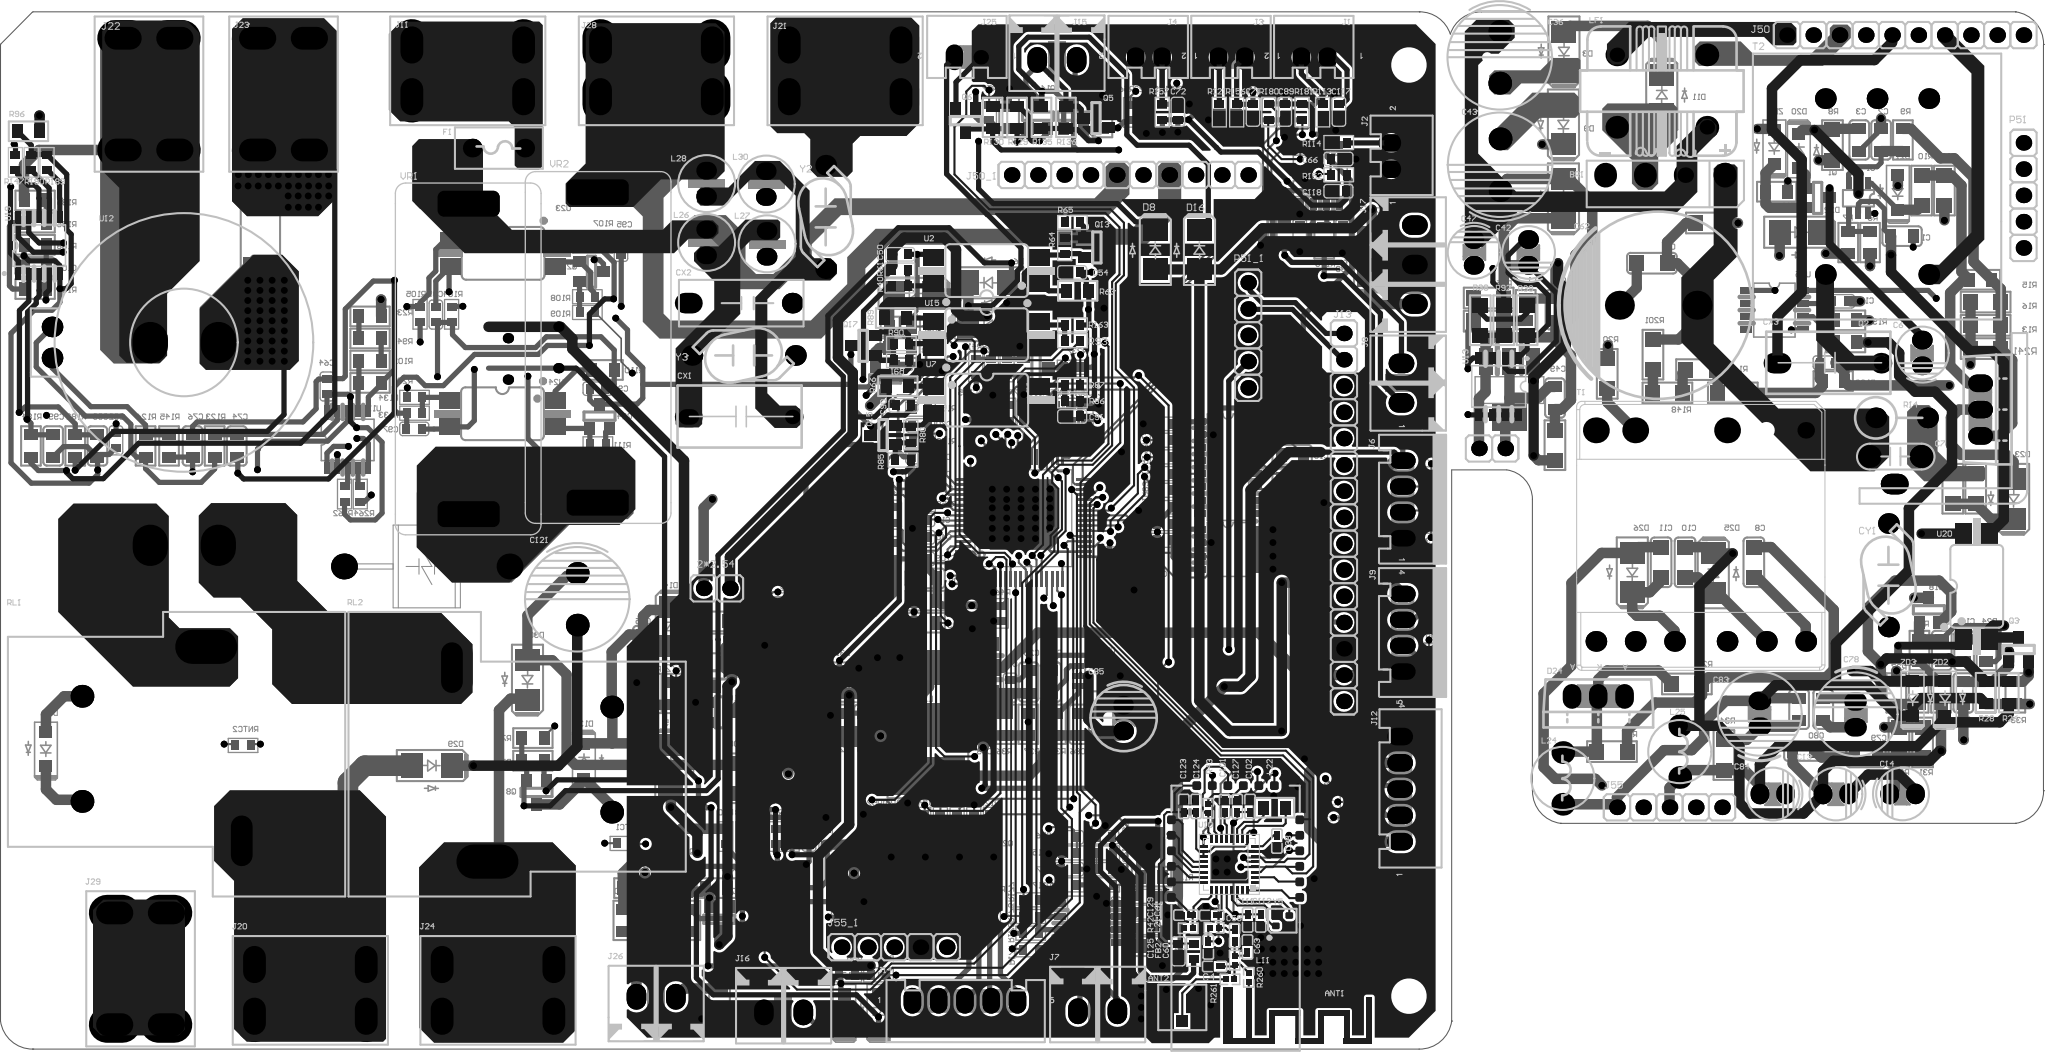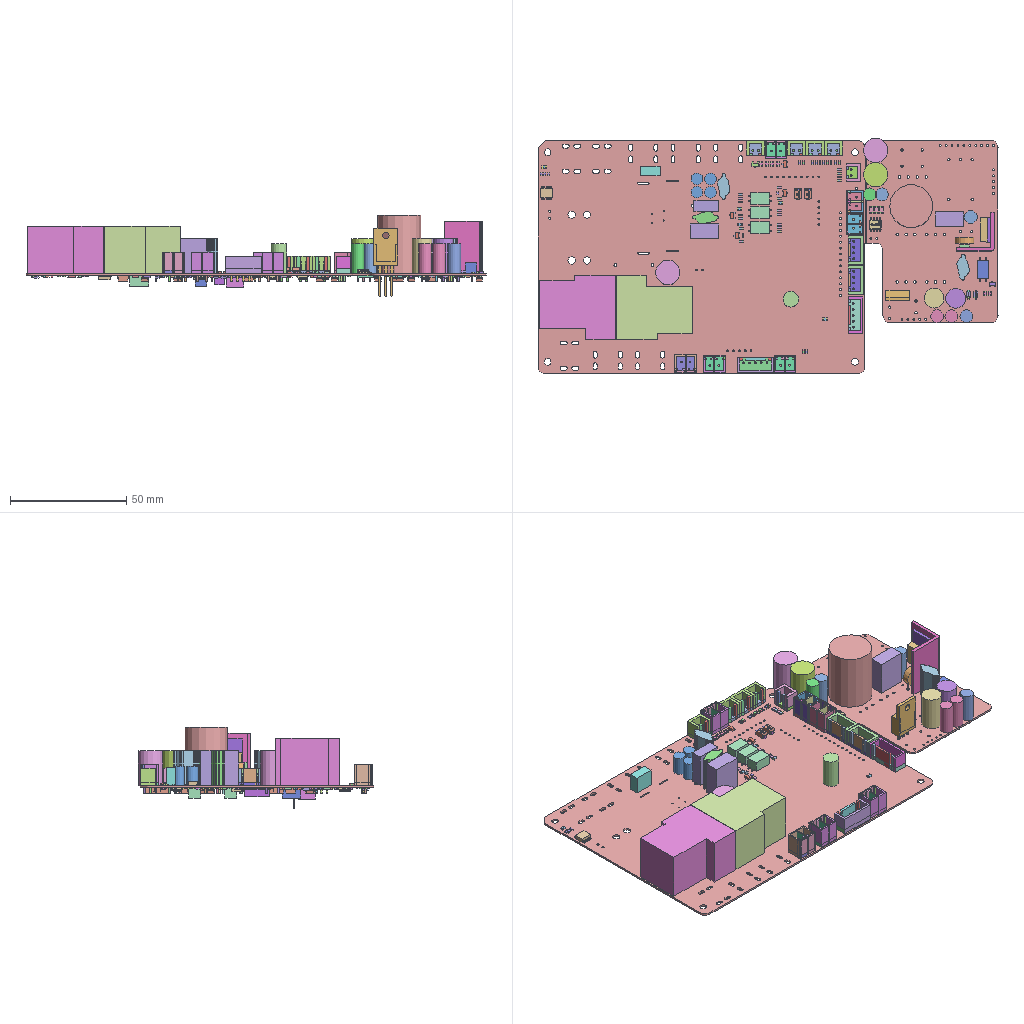Circuit board layout | Altium Designer | box 197.5 x 101.1 x 34.9 mm
Layer stack:
# Altium Designer layer stack of  (unit mm; dielectric type: 0 none, 1 core, 2 prepreg, 3 surface material)
index,name,kind,layer,copper_thickness_mm,dielectric_type,dielectric_thickness_mm,dielectric_material,dielectric_constant
0,Top Paste,other,,,,,,
1,Top Overlay,other,,,,,,
2,Top Solder,dielectric,,,3,0.0102,Solder Resist,3.5
3,Top Layer,copper,Top Layer,0.0356,,,,
4,Dielectric 1,dielectric,,,1,0.254,FR-4,4.2
5,02,copper,02,0.036,,,,
6,Dielectric 6,dielectric,,,2,0.127,,4.2
7,03,copper,03,0.036,,,,
8,Dielectric 5,dielectric,,,1,0.254,,4.2
9,Bottom Layer,copper,Bottom Layer,0.0356,,,,
10,Bottom Solder,dielectric,,,3,0.0102,Solder Resist,3.5
11,Bottom Overlay,other,,,,,,
12,Bottom Paste,other,,,,,,
# drill layer pairs: low layer,high layer
drill_pair,Top Layer,Bottom Layer
Part placement:
Designator,Comment,Layer,Footprint,Center-X(mm),Center-Y(mm),Rotation
,Comment,TopLayer,蓝牙,49.246,-30.063,270
P51_1,(2.54 socket),TopLayer,P5-2.54,50.463,18.866,270
J55_1,(2.54 socket),TopLayer,P5-2.54,16.251,-40.278,0
J50_1,Header -10-2.54,TopLayer,p10-2.54,39.033,34.36,0
2*2.54,Comment,TopLayer,p2-2.54,-0.8962,-5.594,180
,Comment,TopLayer,p2-2.54,74.041,7.925,180
R148,2.4M,BottomLayer,R1206-T,90.985,13.293,180
R241,1.5R,BottomLayer,R1206-T,121.742,17.577,180
R93,100R,TopLayer,R0603-T,33.48,18.339,180
CX2,0.33uF,TopLayer,CX10.0X4.0-P7.5,1.397,21.971,180
C4,0.5pF/50V,TopLayer,C0402-T,47.221,-42.139,180
J13,(2.54 socket),TopLayer,P15-2.54,59.718,1.262,0
Y3,2.2nF/400V,TopLayer,CY7.5X4.7_P10_AI-DS,1.702,16.916,90
Y2,2.2nF/400V,TopLayer,CY7.5X4.7_P10_AI-DS,9.627,30.302,0
J22,Terminal,TopLayer,接线端子（12X9mm）,-55.778,42.175,270
D16,RS1D,TopLayer,SMA,45.745,27.127,90
D8,RS1D,TopLayer,SMA,41.478,27.127,90
D7,RS1D,BottomLayer,SMA,62.182,26.459,270
T2,EFD30,TopLayer,变压器,111.248,33.24,180
U10,TLSR8251,TopLayer,QFN32_5X5MM,48.643,-32.271,180
L1,1mH  DR8*10,BottomLayer,R0805-T,77.289,21.339,90
U26,MAX232,BottomLayer,SO-16-T,48.516,6.114,270
U13,OB222*,TopLayer,SO-8-t,74.676,13.919,180
D11,US1M,BottomLayer,SMA,90.449,42.139,90
D9,MUR406,BottomLayer,SMA,80.924,39.218,270
D4,MUR406,BottomLayer,SMA,80.924,32.075,270
D3,US1M,BottomLayer,SMA,80.975,46.279,270
C47,100uF/16V,TopLayer,CE5-P2.5MM-AI,71.611,26.873,90
C42,10uF/50V,TopLayer,CE5-P2.5MM-AI,78.259,26.873,270
U8,AT403ARC,BottomLayer,so-64-t1,28.755,1.207,270
C43,100uF/25V,TopLayer,CE10-P5.0MM-AI,75.417,35.347,270
C36,10uF/400V,TopLayer,CE10-P5.0MM-AI,74.172,45.731,90
ZD3,12V,TopLayer,SOD-123-T,114.683,-16.219,270
ZD2,6.2V,TopLayer,SOD-123-T,117.808,-16.219,270
ZD1,13V,BottomLayer,SOD-123-T,101.323,37.07,270
ZC1,Discharge tube SE801H-L,BottomLayer,ZC_8X6.5__P:16.0mm,-28.931,-3.48,0
Y5,24MHz,TopLayer,23047-00020-11_32M_SMD¾§Õñ,53.787,-37.716,0
Y1,25MHz,BottomLayer,SMD晶振（HC-49）,12.954,0,270
U25,LM293,BottomLayer,so-8-t,101.323,21.298,270
U24,BPC-1009,BottomLayer,OPT-SMT(LTV-817S),-21.613,11.281,180
U23,BPC-1009,BottomLayer,OPT-SMT(LTV-817S),-21.552,26.784,180
U22,RS485,BottomLayer,SO-8-T,34.996,-37.947,90
U20,LTV-817C,TopLayer,OPT-SMT(LTV-817S),120.881,-5.397,90
U19,BL0942,TopLayer,SO-10-T（脚距1.0mm),-66.396,27.534,0
U18,TL431,BottomLayer,SOT-23((TL431)(A_K_R)-T,116.258,-7.683,180
U17,SM8102H,BottomLayer,SOT-23-6-T,35.514,-14.046,270
U16,AMS1117-3V3,BottomLayer,SOT-223-T,75.717,13.619,0
U15,BPC-1009,TopLayer,OPT-SMT(LTV-817S),25.197,18.923,0
U14,LM2904,BottomLayer,so-8-t,4.32,-37.274,180
U12,CTZ-LB-10,TopLayer,23012-00041-10__µçÁ÷»¥¸ÐÆ÷,-65.149,18.172,270
U11,BL0942,BottomLayer,SO-10-T（脚距1.0mm),-36.574,8.75,0
U9,AT24C16M/TR,BottomLayer,SO-8-t,48.516,-1.839,270
U7,BPC-1009,TopLayer,OPT-SMT(LTV-817S),25.197,12.598,0
U6,TJA1050,BottomLayer,SO-8-T,57.432,34.27,0
U5,AMS1117-3V3,BottomLayer,SOT-223-T,22.358,-13.271,270
U3,TLP785,BottomLayer,OPT-SMT(LTV-817S),4.981,-14.77,90
U2,BPC-1009,TopLayer,OPT-SMT(LTV-817S),25.197,25.118,180
U1,OB2365E,BottomLayer,SOT-23-6-T,109.449,32.101,180
T1,PQ20/20,TopLayer,PQ2020,94.211,-0.5206,0
RNTC2,NTC,BottomLayer,R0603-t,-46.685,-20.777,0
RNTC1,NTC,BottomLayer,R0603-t,-9.779,-30.251,180
RL2,T9VV1K15-12S,TopLayer,继电器（T9VV1K15-12S）,-18.774,-22.632,90
RL1,T9VV1K15-12S,TopLayer,继电器（T9VV1K15-12S）,-54.532,-20.622,270
R264,10K,BottomLayer,R0603-T,-35.354,3.518,90
R263,30K,BottomLayer,R1206-T,6.056,-23.952,90
R261,0R,TopLayer,R0402-T,48.706,-43.384,180
R260,0R,TopLayer,R0402-T,50.523,-43.194,90
R240,10K,BottomLayer,R0603-T,14.731,-42.95,0
R239,10K,BottomLayer,R0603-T,27.162,15.799,90
R238,100R,BottomLayer,R0603-T,25.646,15.799,90
R237,3K,BottomLayer,R0603-T,33.445,15.773,180
R236,100R,BottomLayer,R0603-T,60.792,-24.651,180
R235,100R,BottomLayer,R0603-T,60.792,-26.2,180
R234,100R,BottomLayer,R0603-T,60.792,-27.749,180
R233,10K,BottomLayer,R0603-T,60.792,-23.101,180
R232,1k,BottomLayer,R0805-T,-34.412,14.262,0
R231,1.5M,BottomLayer,R0805-T,-34.412,20.689,0
R214,5.1K,BottomLayer,R0603-T,24.314,-36.541,90
R213,5.1K,BottomLayer,R0603-T,22.79,-36.534,90
R201,2.4M,BottomLayer,R1206-T,89.585,16.993,90
R200,30K,BottomLayer,R1206-T,1.145,-23.952,90
R199,2K,BottomLayer,R0805-T,19.245,-8.915,180
R198,30K,BottomLayer,R1206-T,3.601,-23.952,270
R197,1K,BottomLayer,R0805-T,19.245,-6.782,180
R196,10K,BottomLayer,R0805-T,5.182,-7.391,0
R195,30K,BottomLayer,R1206-T,8.511,-23.952,90
R194,20K,BottomLayer,R0805-T,108.201,18.174,180
R193,1K,BottomLayer,R0805-T,108.201,20.308,0
R192,22K,BottomLayer,R0805-T,107.008,14.44,180
R191,2.4M,BottomLayer,R1206-T,97.307,13.293,180
R190,10K,TopLayer,R0603-T,-67.157,35.579,270
R189,10K,TopLayer,R0603-T,-65.633,35.579,270
R188,1k,BottomLayer,R0805-T,-66.782,27.614,180
R187,1.5M,BottomLayer,R0805-T,-66.782,23.334,180
R186,1.5M,BottomLayer,R0805-T,-66.782,29.754,0
R185,1.5M,BottomLayer,R0805-T,-66.782,31.894,180
R184,1k,BottomLayer,R0805-T,-67.187,8.17,90
R183,1mΩ,BottomLayer,R2512-T,-45.009,28.626,270
R182,1k,BottomLayer,R0805-T,-62.907,8.17,90
R181,100R,TopLayer,R0603-T,55.677,40.437,270
R180,100R,TopLayer,R0603-T,52.451,40.437,90
R179,120R,BottomLayer,R0805-T,57.813,28.185,90
R178,10K,BottomLayer,R0603-T,40.615,-35.36,180
R177,100R,BottomLayer,R0603-T,29.445,-35.703,0
R176,120R,BottomLayer,R0805-T,41.122,-33.455,0
R175,100R,BottomLayer,R0603-T,29.445,-37.312,0
R174,100R,BottomLayer,R0603-T,29.445,-40.529,0
R173,10K,BottomLayer,R0603-T,29.445,-38.92,0
R171,10K,BottomLayer,R0603-T,40.615,-36.884,0
R170,0R,BottomLayer,R0603-T,68.176,4.724,270
R163,4.7K,TopLayer,R0603-T,33.48,19.86,0
R162,10K,BottomLayer,R0603-T,-36.878,3.518,270
R159,NC,BottomLayer,R0603-T,42.171,40.41,90
R158,1K,BottomLayer,R0603-T,18.796,2.514,0
R157,1K,TopLayer,R0603-T,42.16,40.436,270
R156,NC,TopLayer,R0603-T,49.352,40.437,90
R155,1K,BottomLayer,R0603-T,18.796,11.723,0
R154,10K,BottomLayer,R0603-T,50.922,40.437,270
R153,1K,BottomLayer,R0603-T,18.796,8.653,0
R152,10K,TopLayer,R0603-T,59.217,34.377,0
R151,1K,BottomLayer,R0603-T,31.834,11.349,270
R150,10K,BottomLayer,R0603-T,55.667,40.437,270
R149,2.4M,BottomLayer,R1206-T,94.234,15.545,180
R147,10K,TopLayer,R0603-T,-68.681,35.579,90
R145,1.2K,BottomLayer,R0805-T,-53.84,8.17,90
R142,NC,BottomLayer,RES/0603,42.446,7.11,180
R141,NC,BottomLayer,RES/0603,42.446,8.722,180
R140,0R,BottomLayer,R0805-T,68.478,-7.67,90
R139,0R,BottomLayer,R0805-T,68.478,-12.802,270
R137,0R,BottomLayer,R0603-T,68.176,1.161,90
R136,10K,TopLayer,R0805-T,32.849,39.929,270
R135,5.1K,TopLayer,R0805-T,30.487,39.929,270
R134,100R,BottomLayer,R0603-T,-30.112,12.865,0
R133,4.7K,BottomLayer,R0603-T,-30.112,11.334,180
R130,10K,TopLayer,R0805-T,25.762,39.929,90
R129,5.1K,TopLayer,R0805-T,28.124,39.929,90
R128,10K,BottomLayer,R0603-T,23.94,-28.188,90
R127,100R,BottomLayer,R0603-T,25.552,-28.188,90
R126,5.1K,BottomLayer,R0603-T,25.838,-36.541,90
R125,5.1K,BottomLayer,R0603-T,21.271,-36.541,90
R124,1.2k,BottomLayer,R0805-T,-56.109,8.17,90
R123,1.2K,BottomLayer,R0805-T,-49.432,8.17,270
R122,1K,BottomLayer,R0603-T,40.617,40.41,270
R121,1K,TopLayer,R0603-T,47.676,40.437,270
R120,1K,BottomLayer,R0603-T,36.599,-34.255,0
R119,1K,BottomLayer,R0603-T,30.325,11.349,270
R118,10K,BottomLayer,R0603-T,36.599,-31.17,0
R117,1K,BottomLayer,R0603-T,33.181,-34.255,180
R116,1K,BottomLayer,R0603-T,27.306,11.349,270
R115,10K,BottomLayer,R0603-T,33.181,-31.17,180
R114,1K,TopLayer,R0603-T,59.217,37.49,0
R113,1K,TopLayer,R0603-T,57.658,40.437,90
R112,2K,BottomLayer,R0603-T,-12.391,6.845,180
R111,4.7K,BottomLayer,R0603-T,-12.391,8.369,180
R110,300R,BottomLayer,R0805-T,-11.885,15.513,180
R109,2K,BottomLayer,R0603-T,-13.407,21.069,180
R108,4.7K,BottomLayer,R0603-T,-13.407,22.593,0
R107,470R,BottomLayer,R0805-T,-12.901,27.8,0
R105,100R,BottomLayer,R0603-T,-29.578,20.891,270
R104,4.7K,BottomLayer,R0603-T,-26.53,20.891,270
R103,10K,BottomLayer,R0805-T,-8.913,-34.565,0
R102,1.5M,BottomLayer,R0805-T,-34.412,16.421,0
R100,510K,BottomLayer,R0805-T,-9.929,-37.689,90
R99,1K,BottomLayer,R0805-T,-5.611,-37.689,90
R97,1K,BottomLayer,R0805-T,-3.452,-37.689,270
R96,0R,TopLayer,R0805-T,-67.425,38.583,180
R95,1.2K,BottomLayer,R1206-T,80.112,8.243,90
R94,1.5M,BottomLayer,R0805-T,-34.412,18.555,180
R92,390K,TopLayer,R1206-T,75.159,20.32,90
R91,2K,TopLayer,R0603-T,16.942,16.434,0
R90,4.7K,TopLayer,R0603-T,16.942,18.059,0
R89,470R,TopLayer,R0805-T,16.384,20.531,0
R88,2R,BottomLayer,R1206-T,73.707,20.231,180
R87,100R,TopLayer,R0603-T,33.48,14.072,180
R86,4.7K,TopLayer,R0603-T,33.48,12.533,0
R85,2K,TopLayer,R0603-T,17.11,6.807,0
R84,10K,BottomLayer,R0603-T,3.179,-29.584,270
R83,100R,BottomLayer,RES/0603,42.446,3.885,0
R82,10K,BottomLayer,R0603-T,6.386,-29.584,90
R81,10K,BottomLayer,R0603-T,4.783,-29.584,270
R80,4.7K,TopLayer,R0603-T,17.86,9.22,90
R79,1.5K,BottomLayer,R0603-T,11.613,-35.877,180
R78,124K,BottomLayer,R0603-T,1.626,-29.584,270
R77,10K,BottomLayer,R0603-T,11.613,-34.38,0
R75,2K,BottomLayer,R0805-T,-0.9398,-34.565,180
R74,10K,BottomLayer,R0805-T,-18.672,-22.254,180
R73,10K,BottomLayer,R0805-T,-7.186,-15.751,270
R71,470R,BottomLayer,R0805-T,-18.672,-20.067,0
R70,5.1K,BottomLayer,R0805-T,-0.8636,-10.922,180
R69,10K,BottomLayer,R0805-T,-0.889,-8.788,180
R68,10K,BottomLayer,R0805-T,16.815,17.628,180
R67,470R,BottomLayer,R0805-T,16.84,19.71,0
R66,470R,TopLayer,R0805-T,16.603,13.945,0
R65,2K,TopLayer,R0603-T,33.48,29.766,0
R64,4.7K,TopLayer,R0603-T,32.73,27.51,270
R63,470R,TopLayer,R0805-T,33.986,23.162,0
R61,4.7K,TopLayer,R0603-T,16.794,25.167,180
R60,100R,BottomLayer,R0603-T,-0.0281,-29.584,90
R59,10K,BottomLayer,R0805-T,27.358,39.904,270
R58,10K,BottomLayer,R0805-T,36.375,39.904,270
R57,1K,BottomLayer,R0603-T,25.453,40.41,90
R56,1K,BottomLayer,R0603-T,39.093,40.41,270
R55,10K,BottomLayer,R0603-T,11.669,-42.95,180
R54,10K,BottomLayer,R0603-T,42.446,0.6601,0
R53,10K,BottomLayer,R0603-T,42.446,-0.9524,0
R52,10K,BottomLayer,R0603-T,14.267,-28.188,90
R51,100R,BottomLayer,R0603-T,15.879,-28.188,90
R50,10K,BottomLayer,R0603-T,20.715,-28.188,90
R49,10K,BottomLayer,R0603-T,17.491,-28.188,90
R48,100R,BottomLayer,R0603-T,22.328,-28.188,90
R47,100R,BottomLayer,R0603-T,19.103,-28.188,90
R46,10K,BottomLayer,R0603-T,26.594,-8.013,270
R45,2R,BottomLayer,R1206-T,73.707,22.468,180
R44,1M,BottomLayer,R0603-T,8.788,-0.0508,90
R43,1K,TopLayer,R0402-T,46.611,-26.858,270
R42,0R,TopLayer,R0402-T,44.667,-38.445,0
R41,5.1K,BottomLayer,R0603-T,24.131,15.799,90
R40,100R,TopLayer,R0603-T,16.794,23.643,180
R39,390K,TopLayer,R1206-T,77.419,20.32,90
R38,390K,TopLayer,R1206-T,72.898,20.32,270
R37,22K1,BottomLayer,R0805-T,29.212,-18.732,90
R36,100K,BottomLayer,R0805-T,27.053,-18.732,270
R35,10K,BottomLayer,R0805-T,31.879,-18.732,90
R34,N.C,BottomLayer,R1206-T,96.446,-21.704,270
R33,470R,BottomLayer,R0805-T,124.612,-15.697,90
R32,1K1,BottomLayer,R0805-T,121.745,-15.697,270
R31,N.C,BottomLayer,R1206-T,115.649,-20.489,90
R30,N.C,BottomLayer,R1206-T,113.363,-20.489,90
R29,200K,BottomLayer,R0805-T,113.109,-15.702,90
R28,6K8,TopLayer,R0805-T,121.742,-15.672,90
R27,1K8,BottomLayer,R0805-T,115.268,-15.702,90
R26,N.A,TopLayer,R0805-T,123.977,-15.672,90
R25,470R,BottomLayer,R0805-T,117.427,-15.702,90
R24,N.C,BottomLayer,R0805-T,121.821,-11.603,90
R23,22R,BottomLayer,R1206-T,92.865,-14.834,180
R22,22R,BottomLayer,R1206-T,85.626,-21.374,180
R21,4K7,BottomLayer,R0805-T,115.344,-11.603,90
R20,2.2R,BottomLayer,R1206-T,85.166,15.138,270
R19,100R,BottomLayer,R1206-T,120.779,4.035,90
R18,NC,BottomLayer,RES/0603,42.446,5.497,0
R17,100R,BottomLayer,R1206-T,118.57,4.035,90
R16,1.5R,BottomLayer,R1206-T,121.742,22.073,180
R15,10K,BottomLayer,R0805-T,121.242,24.232,0
R14,100K 1W,TopLayer,R-1W-P5.0-V,113.627,10.884,0
R13,1.5R,BottomLayer,R1206-T,121.742,19.825,180
R12,10R,BottomLayer,R1206-T,117.757,32.851,90
R11,10K,BottomLayer,R0805-T,101.547,32.744,180
R10,47R,BottomLayer,R1206-T,115.547,32.851,90
R9,470R,BottomLayer,R0805-T,113.744,37.745,90
R8,220K,BottomLayer,R1206-T,106.936,37.245,90
R7,27K,BottomLayer,R0805-T,108.46,27.825,270
R6,100K,BottomLayer,R0805-T,110.569,27.826,90
R5,220K,BottomLayer,R1206-T,95.185,29.718,0
Q24,MMBT4403LT1G,BottomLayer,SOT-23-T,-12.235,11.036,180
Q23,MMBT4403LT1G,BottomLayer,SOT-23-T,-13.024,25.006,90
Q22,AP2306AGN,BottomLayer,SOT-23-T,29.947,15.723,90
Q21,AP2306AGN,BottomLayer,SOT-23-T,24.917,-31.737,0
Q20,AP2306AGN,BottomLayer,SOT-23-T,15.011,-31.737,0
Q19,AP2306AGN,BottomLayer,SOT-23-T,21.615,-31.737,0
Q18,AP2306AGN,BottomLayer,SOT-23-T,18.313,-31.737,0
Q17,MMBT4403LT1G,TopLayer,SOT-23-T,13.252,17.846,90
Q16,AOSS21311C,BottomLayer,SOT-23-T,33.581,40.027,180
Q15,MMBT4403LT1G,TopLayer,SOT-23-T,15.18,9.22,90
Q14,AOSS21311C,BottomLayer,SOT-23-T,30.152,40.027,180
Q13,MMBT4403LT1G,TopLayer,SOT-23-T,35.826,27.353,270
Q12,LMBT5401LT1G,BottomLayer,SOT-23-T,-4.722,-33.738,180
Q11,LMBT5551LT1G,BottomLayer,SOT-23-T,-0.658,-37.566,0
Q10,AP2306AGN,BottomLayer,SOT-23-T,-0.6604,-17.577,90
Q9,AOSS21311C,BottomLayer,SOT-23-T,-1.016,-13.945,0
Q8,AP2306AGN,BottomLayer,SOT-23-T,-18.322,-25.302,0
Q7,AP2306AGN,BottomLayer,SOT-23-T,15.367,14.656,0
Q6,AP2306AGN,TopLayer,SOT-23-T,23.171,39.626,180
Q5,AP2306AGN,TopLayer,SOT-23-T,35.77,39.853,90
Q3,2N3904,TopLayer,SOT-23-T,124.945,-11.519,0
Q2,4A/650V,TopLayer,TO-220((É¢ÈÈÆ¬16.5X16mm_ºñ1.5mm),117.106,9.353,270
Q1,BC846B,BottomLayer,SOT-23-T,105.489,32.144,90
LF1,18mH,TopLayer,UU9.8_-_(8.7MM),90.449,42.469,0
L31,3.9uH,BottomLayer,R0805-T,10.95,-14.655,90
L30,100uH,TopLayer,71453-00013-11_(5X8.3_P:2.5),3.886,33.483,270
L29,SWCS0503-100MT 10uH/1.8A,BottomLayer,L(8x8x4)-3d,19.507,-21.374,90
L28,100uH,TopLayer,71453-00013-11_(5X8.3_P:2.5),-1.88,33.528,270
L27,100uH,TopLayer,71453-00013-11_(5X8.3_P:2.5),3.962,27.706,270
L26,100uH,TopLayer,71453-00013-11_(5X8.3_P:2.5),-1.88,27.838,270
L25,3.3uH,TopLayer,L-DR6-P5.0,92.179,-21.374,270
L24,3.3uH,TopLayer,L-DR6-P5.0,80.876,-23.965,270
L22,47uH,TopLayer,R0805-T,53.018,-26.797,180
L21,1.3nH,TopLayer,R0402-T,47.166,-38.406,0
L11,3.3nH,TopLayer,R0402-T,49.151,-41.529,90
J29,Terminal,TopLayer,接线端子（12X9mm）,-56.591,-42.367,90
J28,Terminal,TopLayer,接线端子（12X9mm）,-6.731,44.425,0
J26,CON2,TopLayer,CON2-3.81,-6.757,-45.072,180
J25,CON2,TopLayer,con2-2.54,23.345,45.733,180
J24,Terminal,TopLayer,接线端子（12X9mm）,-22.045,-44.452,180
J23,Terminal,TopLayer,接线端子（12X9mm）,-42.774,42.175,270
J21,Terminal,TopLayer,接线端子（12X9mm）,11.506,44.425,0
J20,Terminal,TopLayer,接线端子（12X9mm）,-40.18,-44.452,0
J17,CON3,TopLayer,CON3-3.81,66.576,25.697,90
J16,CON2,TopLayer,CON2-3.81,5.562,-46.582,0
J15,CON2,TopLayer,CON2-3.81,31.981,45.479,0
J14,CON5,TopLayer,CON5-2.54,23.088,-45.453,0
J12,CON5,TopLayer,CON5-2.54,65.153,-25.001,90
J11,Terminal,TopLayer,接线端子（12X9mm）,-24.968,44.425,180
J9,CON4,TopLayer,CON4-2.5,65.407,-9.888,270
J8,CON2,TopLayer,CON2-3.81,65.28,14.242,270
J7,CON2,TopLayer,CON2-3.81,35.915,-46.469,0
J6,CON4,TopLayer,CON4-2.5,65.407,2.999,270
J4,CON2,TopLayer,CON2-2.54,40.871,45.733,180
J3,CON2,TopLayer,CON2-2.54,48.872,45.733,180
J2,CON2,TopLayer,CON2-2.54,64.29,36.187,90
J1,CON2,TopLayer,CON2-2.54,56.873,45.733,180
FB2,BLM15HG102SN1,TopLayer,R0603-T,45.189,-40.703,90
FB1,600Ω/100MHZ,BottomLayer,R1206-T,-0.6326,-45.733,90
F1,T2A/250V,TopLayer,FUSE-TE5,-21.996,36.957,180
D31,1N4148,BottomLayer,SOD-123-T,14.731,-46.482,270
D30,US1M,BottomLayer,SMA-T,-19.202,-14.442,270
D29,US1M,BottomLayer,SMA-T,-28.423,-22.733,0
D26,DSS110,BottomLayer,SMA-T,87.582,-4.072,270
D25,SS16,BottomLayer,SMA-T,95.43,-4.122,90
D24,MBR20100CT,TopLayer,TO-220(AKA二极管）,84.305,-16.04,180
D23,FR107,BottomLayer,SMA-T,124.437,3.035,270
D22,RS1D,BottomLayer,SMA-T,103.736,28.816,0
D21,1N4148,BottomLayer,SOD-123-T,113.261,32.676,270
D20,1N4148,BottomLayer,SOD-123-T,103.685,36.69,90
D19,S545L,BottomLayer,SMA-T,18.136,22.902,0
D17,1N4148,BottomLayer,SOD-123-T,11.429,-46.482,270
D15,S545L,BottomLayer,SMA-T,-5.334,-22.682,90
D14,S545L,BottomLayer,SMA-T,-5.281,-9.263,90
D13,1N4148,BottomLayer,SOD-123-T,-13.741,-22.301,90
D12,1N4148,BottomLayer,SOD-123-T,-65.735,-21.133,270
D10,S545L,BottomLayer,SMA-T,25.324,19.812,180
D6,S545L,BottomLayer,SMA-T,25.324,23.952,180
D5,SESOT12CLC,BottomLayer,SOT-23-T,52.781,28.535,270
D2,SESOT12CLC,BottomLayer,SOT-23-T,40.772,-30.493,0
CX3,2.2nF/275V,TopLayer,CX12.0X6.0-P10,106.628,16.167,180
CX1,2.2nF/275V,TopLayer,CX12.0X6.0-P10,1.397,10.973,180
C129,1uF/50V,TopLayer,C0402-T,44.443,-37.175,180
C127,0.1uF,TopLayer,C0402-T,49.414,-26.671,270
C125,2.2uF/50V,TopLayer,C0603-T,43.716,-40.678,270
C124,1uF,TopLayer,C0402-T,45.441,-26.671,90
C123,1uF,TopLayer,C0402-T,44.24,-26.671,90
C121,6.8uF/400V,TopLayer,CE10-P5.0MM-AI-DS,-14.989,-6.652,90
C120,0.1uF/50V,BottomLayer,C0603-T,106.471,16.218,180
C119,0.1uF/50V,BottomLayer,C0603-T,107.665,22.149,0
C118,0.1uF/50V,TopLayer,C0603-T,59.187,32.79,0
C117,0.1uF/50V,TopLayer,C0603-T,59.233,40.467,90
C116,0.1uF/50V,BottomLayer,C0603-T,33.314,11.379,90
C115,0.1uF/50V,BottomLayer,C0603-T,54.056,40.467,270
C114,1nF/50V,BottomLayer,C0603-T,8.02,-29.614,270
C112,1uF,TopLayer,C0402-T,51.668,-37.649,270
C111,0.1uF,TopLayer,C0402-T,50.413,-37.649,270
C110,20pF/50V,BottomLayer,C0603-T,16.307,-1.988,270
C109,0.1uF/50V,BottomLayer,C0603-T,18.766,-2.756,0
C108,10uF/10V,BottomLayer,C0805-T,19.245,-4.635,180
C107,10uF/10V,BottomLayer,C0805-T,38.357,-4.089,0
C106,0.1uF/50V,BottomLayer,C0603-T,37.821,-2.235,0
C105,0.1uF/50V,BottomLayer,C0603-T,24.257,11.379,90
C104,0.1uF/50V,BottomLayer,C0603-T,25.121,-7.983,270
C103,0.1uF/50V,BottomLayer,C0603-T,34.823,11.379,90
C102,2.2uF,TopLayer,C0402-T,50.642,-26.671,270
C101,1uF,TopLayer,C0402-T,48.184,-26.671,90
C100,33nF,BottomLayer,C0805-T,-66.782,25.468,180
C99,33nF,BottomLayer,C0805-T,-65.047,8.17,90
C98,33nF,BottomLayer,C0805-T,-60.761,8.17,270
C97,0.1uF/50V,BottomLayer,C0603-T,-30.142,9.817,180
C96,0.1uF/50V,BottomLayer,C0603-T,-12.421,13.703,0
C95,0.1uF/50V,BottomLayer,C0603-T,-10.16,27.407,270
C93,0.1uF/50V,BottomLayer,C0603-T,-28.054,20.861,270
C92,0.1uF/50V,BottomLayer,C0603-T,-58.964,8.706,270
C91,0.1uF/50V,TopLayer,C0603-T,33.45,11.024,0
C90,0.1uF/50V,TopLayer,C0603-T,17.14,12.09,180
C89,15pF/50V,TopLayer,C0603-T,54,40.467,270
C88,15pF/50V,BottomLayer,C0603-T,59.591,28.721,270
C87,0.1uF,BottomLayer,C0805-T,103.711,-17.285,90
C86,0.1uF,BottomLayer,C0805-T,34.115,-18.732,270
C85,22u/50V,TopLayer,CE6.3-P2.5MM-AI-DS,37.738,-18.135,90
C84,100uF/16V,TopLayer,CE5-P2.5MM-AI-DS,101.17,-24.781,0
C83,470uF/25V,TopLayer,CE8-P2.5MM-AI-DS,100.611,-17.716,270
C82,10nF,BottomLayer,C0805-T,119.586,-15.702,270
C81,0.1uF,BottomLayer,C0805-T,106.047,-17.285,270
C80,0.1uF,BottomLayer,C0805-T,104.168,-21.315,180
C79,0.1uF,BottomLayer,C0805-T,110.178,-21.939,180
C78,680uF/25V,TopLayer,CE8-P2.5MM-AI-DS,108.484,-17.773,90
C77,0.1uF/50V,BottomLayer,C0603-T,43.665,40.44,270
C76,33nF,BottomLayer,C0805-T,-51.566,8.17,270
C74,33nF,BottomLayer,C0805-T,-47.292,8.17,90
C73,0.1uF/50V,BottomLayer,C0603-T,18.766,4.019,180
C72,0.1uF/50V,TopLayer,C0603-T,43.663,40.466,270
C71,0.1uF/50V,TopLayer,C0603-T,50.927,40.467,270
C70,0.1uF/50V,BottomLayer,C0603-T,18.766,10.158,180
C69,0.1uF/50V,BottomLayer,C0603-T,36.569,-29.658,0
C68,0.1uF/50V,BottomLayer,C0603-T,52.474,40.467,270
C67,0.1uF/50V,BottomLayer,C0603-T,33.151,-32.742,180
C66,0.1uF/50V,TopLayer,C0603-T,59.187,35.904,0
C65,0.1uF/50V,BottomLayer,C0603-T,18.766,7.089,180
C64,0.1uF/50V,BottomLayer,C0603-T,-38.583,13.919,90
C63,2pF/50V,TopLayer,C0402-T,50.396,-40.26,270
C62,47uF/400V,TopLayer,CE18,90.094,21.768,180
C61,2.7pF/50V,TopLayer,C0402-T,46.942,-37.212,0
C60,18pF/50V,TopLayer,C0402-T,46.611,-40.26,90
C59,220pF/50V,TopLayer,C0402-T,49.151,-39.156,90
C58,0.1uF/50V,BottomLayer,C0603-T,36.569,-32.742,180
C57,0.1uF/50V,BottomLayer,C0603-T,28.785,11.379,90
C56,0.1uF/50V,BottomLayer,C0603-T,33.151,-29.658,0
C55,0.1uF/50V,BottomLayer,C0603-T,25.767,11.379,90
C54,0.1uF/50V,TopLayer,C0603-T,33.45,24.94,180
C51,NC,BottomLayer,C0805-T,-7.77,-37.689,90
C50,0.1uF/50V,TopLayer,C0603-T,16.823,26.691,180
C49,1uF/25V/0805,BottomLayer,C0805-T,80.112,12.802,90
C48,0.1uF/50V,BottomLayer,C0603-T,11.583,-37.401,0
C46,0.1uF/50V,BottomLayer,C0603-T,9.624,-29.614,270
C45,0.1uF/50V,BottomLayer,C0805-T,-8.026,-11.127,270
C44,1uF/25V,BottomLayer,C0805-T,80.162,21.339,90
C41,0.1uF/50V,BottomLayer,C0603-T,42.416,2.243,0
C40,0.1uF/50V,BottomLayer,C0603-T,18.766,-0.6621,180
C39,20pF/50V,BottomLayer,C0603-T,16.307,1.524,270
C38,1uF/50V,TopLayer,C0402-T,53.238,-30.023,90
C37,0.1uF/50V,BottomLayer,C0603-T,18.766,5.554,0
C33,47pF,BottomLayer,C0805-T,24.894,-18.732,270
C32,0.1uF/50V,BottomLayer,C0603-T,12.83,-15.191,90
C31,10uF/10V,BottomLayer,C0805-T,14.633,-14.655,90
C30,10uF/10V,BottomLayer,C0805-T,13.332,-18.732,90
C29,10uF/10V,BottomLayer,C0805-T,16.792,-14.655,90
C28,10uF/10V,BottomLayer,C0805-T,11.173,-18.732,90
C27,0.1uF,BottomLayer,C0805-T,31.422,-14.655,270
C26,0.1uF/50V,BottomLayer,C0603-T,27.46,-15.191,90
C25,10uF/10V,BottomLayer,C0805-T,29.238,-14.655,90
C24,15pF/50V,BottomLayer,C0603-T,55.448,28.721,90
C23,1uF/50V,BottomLayer,CAP/0805,54.714,2.558,180
C22,0.1uF/50V,BottomLayer,C0603-T,40.586,-38.408,0
C21,10uF/10V,BottomLayer,C0805-T,41.122,-40.186,0
C20,0.1uF/50V,BottomLayer,CAP/0603,42.416,10.305,180
C19,1uF/50V,BottomLayer,CAP/0805,54.712,5.017,0
C18,1uF/50V,BottomLayer,CAP/0805,54.712,7.318,0
C17,1uF/50V,BottomLayer,CAP/0805,54.712,9.627,180
C15,0.1uF/50V,BottomLayer,C0603-T,18.766,1.025,180
C14,100uF/16V,TopLayer,CE5-P2.5MM-AI-DS,113.718,-26.156,180
C13,100uF/16V,TopLayer,CE5-P2.5MM-AI-DS,107.267,-24.781,0
C12,N.C,BottomLayer,C0805-T,119.662,-11.603,270
C11,n.c,BottomLayer,C1206-T,90.376,-3.072,90
C10,n.c,BottomLayer,C1206-T,92.687,-3.072,90
C9,0.1uF,BottomLayer,C0805-T,117.503,-11.603,270
C8,102/1KV,BottomLayer,C1206-T,99.339,-3.072,90
C7,222/1KV,TopLayer,CC7.5-P5.0MM-AI-2.5-DS,113.007,7.15,180
C6,22uF/50V,TopLayer,CE5-P2.5MM-AI-DS,116.316,17.157,270
C5,10nF/1KV,BottomLayer,C1206-T,89.484,25.832,180
C3,0.1uF,BottomLayer,C0805-T,109.527,37.745,270
C2,100pF,BottomLayer,C0805-T,111.635,37.745,90
C1,1nF,BottomLayer,C0805-T,113.665,28.448,0
BR1,KBJ2J,TopLayer,BD15.22X4.5(KBP206£©RS-2,90.785,34.341,180
ANT2,ANT_SMA,TopLayer,ATN-1,44.094,-46.673,90
ANT1,PCB onboard antenna,TopLayer,ATN,49.513,-44.882,0
CY1,2.2n,TopLayer,CY7.5X4.7_P10_AI-DS,112.347,-4.331,0
R72,470R,BottomLayer,R0805-T,-5.027,-15.751,270
D555,RS1D,BottomLayer,SMA,55.882,-6.942,270
J50,Header -10-2.54,TopLayer,p10-2.54,113.97,47.879,0
J55,(2.54 socket),TopLayer,P5-2.54,91.188,-26.759,0
VR1,TFMOV10M250,TopLayer,防雷单元TFMOV10M,-22.982,16.58,270
VR2,TFMOV10M250,TopLayer,防雷单元TFMOV10M,-14.305,17.685,90
P51,(2.54 socket),TopLayer,P5-2.54,125.4,32.385,270
Pad and via stacks, first 68 of 111 lines:
# Altium Designer via and pad stacks of  (unit mm). Each distinct definition once, with the count of objects using it.
# via: kind,start_layer,end_layer,hole_mm,diameter_mm,mode(0 simple;1 top-mid-bottom;2 full stack),diameter_per_layer,count,example_net
# pad: kind,layer,hole_mm,hole_type(0 round;1 square;2 slot),plating,top_size,top_shape(1 round;2 rect;3 octagon;9 rounded rect),mid_size,bottom_size,mode,footprint,size_per_layer,count,example
pad,Multi-Layer,1,0,plated,2x2,1,2x2,2x2,0,23012-00041-10  \u00B5\u00E7\u00C1\u00F7\u00BB\u00A5\u00B8\u00D0\u00C6\u00F7,,2,U12.2
pad,Multi-Layer,3.2,0,plated,4x3.4,1,4x3.4,4x3.4,0,,,4,1
pad,Multi-Layer,1,2,plated,2x1.5,1,2x1.5,2.7x2,1,CX12.0X6.0-P10,,2,CX3.2
pad,Multi-Layer,1,0,plated,1.4x1.4,1,1.4x1.4,2x2,1,CX12.0X6.0-P10,,2,CX3.1
pad,Multi-Layer,1,0,plated,1.7x2.4,1,1.7x2.4,1.7x2.4,0,TO-220((\u00C9\u00A2\u00C8\u00C8\u00C6\u00AC16.5X16mm \u00BA\u00F11.5mm),,3,Q2.1
pad,Multi-Layer,1.2,2,plated,2.7x2,1,2.7x2,2.7x2,0,TO-220((\u00C9\u00A2\u00C8\u00C8\u00C6\u00AC16.5X16mm \u00BA\u00F11.5mm),,1,Q2.0
pad,Multi-Layer,1,0,plated,1.8x2,1,1.8x2,1.8x2,0,CE5-P2.5MM-AI-DS,,4,C13.1
pad,Multi-Layer,1,0,plated,2x1.8,1,2x1.8,2x1.8,0,CE5-P2.5MM-AI-DS,,4,C13.2
pad,Multi-Layer,0.7,0,unplated,0x0,1,0x0,0x0,0,CE5-P2.5MM-AI-DS,,4,C13.0
pad,Multi-Layer,1.1,0,plated,2x2,1,2x2,2x2,0,PQ2020,,6,T1.9
pad,Multi-Layer,1.1,0,plated,0x0,1,0x0,0x0,0,PQ2020,,2,T1.2
pad,Multi-Layer,1.1,0,plated,1.6x1.6,1,1.5x1.5,2.5x2.5,1,PQ2020,,4,T1.6
pad,Multi-Layer,1.6,2,plated,2.2x3.6,1,3.5x5,3.5x5,1,\u00BD\u00D3\u00CF\u00DF\u00B6\u00CB\u00D7\u00D3\u00A3\u00A812X9mm\u00A3\u00A9,,24,J20.1
pad,Multi-Layer,1.6,2,plated,3.6x2.2,1,5x3.5,5x3.5,1,\u00BD\u00D3\u00CF\u00DF\u00B6\u00CB\u00D7\u00D3\u00A3\u00A812X9mm\u00A3\u00A9,,8,J20.1
pad,Multi-Layer,1.7,2,plated,4.9x2.1,1,4.9x2.1,6.8x4,1,\u00BC\u00CC\u00B5\u00E7\u00C6\u00F7\u00A3\u00A8T9VV1K15-12S\u00A3\u00A9,,2,RL2.4
pad,Multi-Layer,1.3,2,plated,3.3x6,1,3.3x6,3.3x6,0,\u00BC\u00CC\u00B5\u00E7\u00C6\u00F7\u00A3\u00A8T9VV1K15-12S\u00A3\u00A9,,2,RL2.1
pad,Multi-Layer,1.2,0,plated,2.2x2.2,1,2.2x2.2,2.2x2.2,0,\u00BC\u00CC\u00B5\u00E7\u00C6\u00F7\u00A3\u00A8T9VV1K15-12S\u00A3\u00A9,,4,RL2.2
pad,Multi-Layer,1.1,0,plated,1.9x2.5,1,1.9x2.5,1.9x2.5,0,CON2-3.81,,10,J26.2
pad,Multi-Layer,1,0,plated,1.8x2,1,1.8x2,1.8x2,0,CE6.3-P2.5MM-AI-DS,,1,C85.1
pad,Multi-Layer,1,0,plated,2x1.8,1,2x1.8,2x1.8,0,CE6.3-P2.5MM-AI-DS,,1,C85.2
pad,Multi-Layer,0.7,0,unplated,0x0,1,0x0,0x0,0,CE6.3-P2.5MM-AI-DS,,1,C85.0
pad,Multi-Layer,1,0,plated,1.7x2.5,1,1.7x2.5,1.7x2.5,0,CON5-2.54,,10,J14.1
pad,Multi-Layer,0.8,0,plated,1.5x1.5,1,1.5x1.5,1.5x1.5,0,P5-2.54,,20,P51_1.5
pad,Multi-Layer,0.8,0,plated,1.5x1.5,1,1.5x1.5,1.5x1.5,0,p10-2.54,,20,J50_1.1
pad,Multi-Layer,0.8,0,plated,1.5x1.5,1,1.5x1.5,1.5x1.5,0,p2-2.54,,4,2*2.54.2
pad,Multi-Layer,1.1,0,plated,2x2,1,1.5x1.5,2x2,1,CY7.5X4.7_P10_AI-DS,,6,Y3.2
pad,Multi-Layer,1,0,plated,1.4x1.4,1,1.4x1.4,1.7x2.5,1,con2-2.54,,10,J25.1
pad,Multi-Layer,1.1,0,plated,2.2x2.2,1,2.2x2.2,2.2x2.2,0,CE10-P5.0MM-AI-DS,,2,C121.2
pad,Multi-Layer,0.7,0,unplated,0x0,1,0x0,0x0,0,CE10-P5.0MM-AI-DS,,1,C121.0
pad,Multi-Layer,0.9,0,plated,1.7x2,1,1.3x1.3,1.7x2,1,71453-00013-11 (5X8.3 P:2.5),,8,L26.1
pad,Multi-Layer,1,0,plated,2x2,1,2x2,2x2,0,CX10.0X4.0-P7.5,,1,CX2.1
pad,Multi-Layer,1,2,plated,1.9x1.4,1,1.9x1.4,2.7x2,1,CX10.0X4.0-P7.5,,1,CX2.2
pad,Multi-Layer,0.6,2,plated,2.5x6,9,2.5x6,2.5x6,0,\u00B7\u00C0\u00C0\u00D7\u00B5\u00A5\u00D4\u00AATFMOV10M,,4,VR2.1
pad,Multi-Layer,0.5,0,plated,1x1,1,1x1,1x1,0,\u00B7\u00C0\u00C0\u00D7\u00B5\u00A5\u00D4\u00AATFMOV10M,,4,VR2.4
pad,Multi-Layer,0.9,0,plated,1.8x1.8,1,1.8x1.8,1.8x1.8,0,FUSE-TE5,,2,F1.1
pad,Multi-Layer,0.9,0,plated,2.5x1.6,1,2.5x1.6,2.5x1.6,0,CON4-2.5,,8,J9.4
pad,Multi-Layer,0.8,0,plated,1.5x1.5,1,1.5x1.5,1.5x1.5,0,P15-2.54,,15,J13.15
pad,Multi-Layer,1.1,0,plated,1.9x2.5,1,1.9x2.5,1.9x2.5,0,CON3-3.81,,3,J17.3
pad,Multi-Layer,0.9,0,plated,2x2,1,1.3x1.3,2x2,1,R-1W-P5.0-V,,2,R14.1
pad,Multi-Layer,1.1,0,plated,2.2x2.2,1,1.5x1.5,2.2x2.2,1,CC7.5-P5.0MM-AI-2.5-DS,,2,C7.1
pad,Multi-Layer,1.1,0,plated,1.5x1.5,1,1.5x1.5,2.2x1.8,1,CE8-P2.5MM-AI-DS,,4,C78.1
pad,Multi-Layer,0.7,0,unplated,0x0,1,0x0,0x0,0,CE8-P2.5MM-AI-DS,,2,C78.0
pad,Multi-Layer,1,0,plated,1.4x1.4,1,1.4x1.4,2.2x2.2,1,L-DR6-P5.0,,4,L25.2
pad,Multi-Layer,1.1,0,plated,1.5x1.5,1,1.5x1.5,1.8x2.4,1,TO-220(AKA\u00B6\u00FE\u00BC\u00AB\u00B9\u00DC\u00A3\u00A9,,3,D24.2
pad,Multi-Layer,0.7,0,unplated,0x0,1,0x0,0x0,0,CE5-P2.5MM-AI,,2,C42.0
pad,Multi-Layer,1,0,plated,2x1.8,1,2x1.8,2x1.8,0,CE5-P2.5MM-AI,,2,C42.2
pad,Multi-Layer,1,0,plated,1.8x2,1,1.8x2,1.8x2,0,CE5-P2.5MM-AI,,2,C42.1
pad,Multi-Layer,1.2,0,plated,1.8x1.8,1,1.8x1.8,2.8x2.8,1,CE18,,1,C62.2
pad,Multi-Layer,1.2,0,plated,2.8x2.8,1,2.8x2.8,2.8x2.8,0,CE18,,1,C62.1
pad,Multi-Layer,1.1,0,plated,1.5x1.5,1,2.4x2.2,2.4x2.2,1,BD15.22X4.5(KBP206\u00A3\u00A9RS-2,,2,BR1.3
pad,Multi-Layer,1.1,0,plated,1.5x1.5,1,2.2x2.4,2.2x2.4,1,BD15.22X4.5(KBP206\u00A3\u00A9RS-2,,1,BR1.2
pad,Multi-Layer,1.1,0,plated,2.4x2.2,1,2.4x2.2,2.4x2.2,0,BD15.22X4.5(KBP206\u00A3\u00A9RS-2,,1,BR1.1
pad,Multi-Layer,0.7,0,unplated,0x0,1,0x0,0x0,0,CE10-P5.0MM-AI,,2,C43.0
pad,Multi-Layer,1.1,0,plated,2.2x2.2,1,2.2x2.2,2.2x2.2,0,CE10-P5.0MM-AI,,4,C43.1
pad,Multi-Layer,1,0,plated,1.4x1.4,1,1.4x1.4,2.2x2.2,1,UU9.8 - (8.7MM),,4,LF1.4
pad,Multi-Layer,1,0,plated,2x2,1,2x2,2x2,0,\u00B1\u00E4\u00D1\u00B9\u00C6\u00F7,,5,T2.4
pad,Multi-Layer,1.2,0,plated,2.5x2.5,1,2.5x2.5,2.5x2.5,0,ZC 8X6.5  P:16.0mm,,1,ZC1.1
pad,Multi-Layer,1.2,0,plated,2.5x2.5,1,1.6x1.6,1.6x1.6,1,ZC 8X6.5  P:16.0mm,,1,ZC1.2
pad,Bottom Layer,0,0,plated,1x1.27,2,1x1.27,1x1.27,0,C0805-T,,60,C49.2
pad,Bottom Layer,0,0,plated,1x1.27,2,1x1.27,1x1.27,0,R0805-T,,114,L1.1
pad,Bottom Layer,0,0,plated,1.4x1.525,2,1.4x1.525,1.4x1.525,0,R1206-T,,54,R95.1
pad,Bottom Layer,0,0,plated,1.4x1.5,2,1.4x1.5,1.4x1.5,0,C1206-T,,4,C8.2
pad,Bottom Layer,0,0,plated,1.4x1.524,2,1.4x1.524,1.4x1.524,0,C1206-T,,4,C8.1
pad,Bottom Layer,0,0,plated,2.4x2.1,2,2.4x2.1,2.4x2.1,0,SMA-T,,11,D25.2
pad,Bottom Layer,0,0,plated,2.1x2.4,2,2.1x2.4,2.1x2.4,0,SMA-T,,11,D25.1
Copper pours:
name,layer,net,type(0 solid;1 hatched;2 none)
EARTH_L04_P329,Bottom Layer,EARTH,0
N2_L04_P321,Bottom Layer,N2,0
L-PLC_L04_P319,Bottom Layer,L-PLC,0
-_L04_P281,Bottom Layer,-,0
N-3_L04_P252,Bottom Layer,N-3,0
NETC36_1_L04_P244,Bottom Layer,NetC36_1,0
12VA_L04_P240,Bottom Layer,12VA,0
L1_L04_P230,Bottom Layer,L1,0
ACL-IN_L04_P224,Bottom Layer,ACL-IN,0
NETJP1_2_L04_P172,Bottom Layer,NetJP1_2,0
NETJP2_2_L04_P170,Bottom Layer,NetJP2_2,0
N2_L04_P198,Bottom Layer,N2,0
L-PLC_L04_P184,Bottom Layer,L-PLC,0
L2_L04_P174,Bottom Layer,L2,0
ACL-OUT_L04_P146,Bottom Layer,ACL-OUT,0
IP2_L04_P132,Bottom Layer,IP2,0
ACN-IN_L04_P118,Bottom Layer,ACN-IN,0
ACN-OUT_L04_P116,Bottom Layer,ACN-OUT,0
NETVR1_1_L04_P044,Bottom Layer,NetVR1_1,0
NETC7_1_L04_P006,Bottom Layer,NetC7_1,0
EARTH_L04_P301,Bottom Layer,EARTH,0
-_L01_P345,Top Layer,-,0
-_L01_P341,Top Layer,-,0
-_L01_P339,Top Layer,-,0
EARTH_L01_P331,Top Layer,EARTH,0
EARTH_L01_P323,Top Layer,EARTH,0
Top Layer-NetCX1_1,Top Layer,NetCX1_1,0
NETCX1_2_L01_P277,Top Layer,NetCX1_2,0
L-3_L01_P254,Top Layer,L-3,0
N_L01_P246,Top Layer,N,0
N2_L01_P234,Top Layer,N2,0
NETCX3_1_L01_P232,Top Layer,NetCX3_1,0
+311V_L01_P228,Top Layer,+311V,0
NETJP2_2_L01_P210,Top Layer,NetJP2_2,0
NETJP1_2_L01_P208,Top Layer,NetJP1_2,0
NETVR1_1_L01_P202,Top Layer,NetVR1_1,0
L2_L01_P176,Top Layer,L2,0
ACN-OUT_L01_P156,Top Layer,ACN-OUT,0
ACL-OUT_L01_P154,Top Layer,ACL-OUT,0
IP2_L01_P138,Top Layer,IP2,0
ACN-IN_L01_P126,Top Layer,ACN-IN,0
ACL-IN_L01_P120,Top Layer,ACL-IN,0
L-PLC_L01_P291,Top Layer,L-PLC,0
N2_L01_P293,Top Layer,N2,0
L-PLC_L01_P311,Top Layer,L-PLC,0
-_L03_P347,03,-,0
EARTH_L03_P337,03,EARTH,0
EARTH_L03_P327,03,EARTH,0
L-3_L03_P307,03,L-3,0
N-3_L03_P305,03,N-3,0
03-GND,03,GND,0
-_L03_P260,03,-,0
NETJP2_2_L03_P214,03,NetJP2_2,0
NETJP1_2_L03_P212,03,NetJP1_2,0
L2_L03_P180,03,L2,0
ACN-OUT_L03_P164,03,ACN-OUT,0
ACL-OUT_L03_P162,03,ACL-OUT,0
IP2_L03_P134,03,IP2,0
ACL-IN_L03_P130,03,ACL-IN,0
ACN-IN_L03_P128,03,ACN-IN,0
L-PLC_L03_P283,03,L-PLC,0
N2_L03_P285,03,N2,0
NETVR1_1_L03_P297,03,NetVR1_1,0
-_L02_P349,02,-,0
-_L02_P343,02,-,0
EARTH_L02_P335,02,EARTH,0
EARTH_L02_P325,02,EARTH,0
NETJP2_2_L02_P222,02,NetJP2_2,0
NETJP1_2_L02_P220,02,NetJP1_2,0
02-GND,02,GND,0
-_L02_P262,02,-,0
L2_L02_P178,02,L2,0
ACN-OUT_L02_P160,02,ACN-OUT,0
ACL-OUT_L02_P158,02,ACL-OUT,0
ACN-IN_L02_P140,02,ACN-IN,0
IP2_L02_P136,02,IP2,0
ACL-IN_L02_P122,02,ACL-IN,0
L-PLC_L02_P287,02,L-PLC,0
N2_L02_P289,02,N2,0
NETVR1_1_L02_P295,02,NetVR1_1,0
ACL-OUT_L02_P158,Bottom Solder,ACL-OUT,0
ACN-OUT_L02_P160,Bottom Solder,ACN-OUT,0
EARTH_L02_P325,Bottom Solder,EARTH,0
NETVR1_1_L04_P044,Bottom Solder,NetVR1_1,0
NETJP2_2_L04_P170,Bottom Solder,NetJP2_2,0
NETJP1_2_L04_P172,Bottom Solder,NetJP1_2,0
ACN-IN_L04_P118,Bottom Solder,ACN-IN,0
IP2_L04_P132,Bottom Solder,IP2,0
L2_L04_P174,Bottom Solder,L2,0
L-PLC_L04_P184,Bottom Solder,L-PLC,0
N2_L04_P198,Bottom Solder,N2,0
ACL-IN_L04_P224,Bottom Solder,ACL-IN,0
EARTH_L04_P301,Bottom Solder,EARTH,0
Design rules, without the lines most boards share:
# Altium Designer design rules of  (exported by Altium Designer, unit mm)
# columns: name | kind | enabled | priority | scope1 | scope2 | descriptor | typed fields (field=value)
HoleToHoleClearance | 52 | enabled | 1 | All | All | Hole To Hole Clearance (Gap=10mil) (All),(All) | gap=0.254
DiffPairsRouting | 51 | enabled | 1 | All | All | Differential Pairs Uncoupled Length using the Gap Constraints (Min=10mil) (Max=10mil) (Prefered=10mil)  and Width Constraints (Min=15mil) (Max=15mil) (Prefered=15mil) (All) |
SolderMaskExpansion | 13 | enabled | 1 | All | All | Solder Mask Expansion (Expansion =4mil) (All) | expansion=0.1016
RoutingVias | 11 | enabled | 1 | All | All | Routing Via (MinHoleWidth=1mil) (MaxHoleWidth=50mil) (PreferredHoleWidth=13mil) (MinWidth=1mil) (MaxWidth=50mil) (PreferedWidth=26mil) (All) | via_min_hole=0.0254 via_max_hole=1.27 via_preferred_diameter=0.6604 via_preferred_hole=0.3302
Width | 2 | enabled | 1 | All | All | Width Constraint (Min=6mil) (Max=500mil) (Preferred=8mil) (All) |
PolygonConnect | 20 | enabled | 1 | All | All | Polygon Connect Rule(Direct Connect )(Conductor Width=10mil) (Relief Angle=90 Angle) (Entries=4) (Air Gap Width=10mil) (All),(All) | connect_style(0=relief,1=direct,2=none)=1 relief_conductor_width=0.254 relief_entries=4
PlaneConnect | 6 | enabled | 1 | All | All | Power Plane Connect Rule(NoConnect Connect )(Expansion=20mil) (Conductor Width=10mil) (Air Gap=10mil) (Entries=4) (All) | relief_conductor_width=0.254 relief_entries=4 relief_expansion=0.508
Clearance | 0 | enabled | 1 | All | All | Clearance Constraint (Gap=6mil) (All),(All) | gap=0.1524
Classes set for this board:
# Altium Designer classes of  (member kind: 0 net, 1 component, 2 from-to, 3 pad, 4 layer, 5 differential pair, 6 design channel, 7 polygon, 8 structure, 9 xSignal)
# columns: class name | member kind | superclass | members
RELAY_V0.1 | 1 | no | C15; C45; C46; C48; C51; C114; C119; C120; C121; D6; D10; D12; D13; D14; D15; D19; D29; D30; FB1; J20; J21; J23; J24; J25; J26; J29; Q7; Q8; Q9; Q10; Q11; Q12; R60; R67; R68; R69; R70; R71; R73; R74; R75; R77; R78; R79; R81; R82; R84; R97; R99; R100; R103; R149; R183; R191; R192; R193; R194; R195; R196; R197; R198; R199; R200; R201; R263; RL1; RL2; U3; U14; U25; J22; R72; R148;
POWER_V0.1 | 1 | no | BR1; C1; C2; C3; C5; C6; C7; C8; C9; C10; C11; C12; C13; C14; C25; C26; C27; C28; C29; C30; C31; C32; C33; C36; C42; C43; C44; C47; C49; C62; C78; C79; C80; C81; C82; C83; C84; C85; C86; C87; CX1; CX3; D3; D4; D9; D11; D20; D21; D22; D23; D24; D25; D26; F1; J11; J17; J28; L1; L24; L25; L26; L27; L28; L29; L30; L31; LF1; Q1; Q2; Q3; R5; R6; R7; R8; R9; R10; R11; R12; R13; R14; R15; R16; R17; R19; R20; R21; R22; R23; R24; R25; R26; R27; R28; R29; R30; R31; R32; R33; R34; R35; R36; R37; R38; R39; R45; R88; R92; R95; T1; U1; U5; U13; U16; U17; U18; U20; ZC1; ZD1; ZD2; ZD3; C36; C43; C42; C47; D3; D4; D9; D11; U13; L1; T2; T2; D7; CY1; Y2; Y3; J50; J55; VR1; VR2; CX2; R241; P51;
MCU Controller for 7KW_V0.1 | 1 | no | C37; C39; C40; C41; C103; C104; C105; C106; C107; C108; C109; C110; D17; D31; J12; J14; J16; Q18; Q19; Q20; Q21; Q22; R41; R44; R46; R47; R48; R49; R50; R51; R52; R53; R54; R55; R125; R126; R127; R128; R213; R214; R233; R234; R235; R236; R237; R238; R239; R240; U9; Y1; U8; J13; D555;
ElectricLeakage-Check_V0.1 | 1 | no | C50; C54; C64; C74; C76; C90; C91; C92; C93; C95; C96; C97; C98; C99; C100; Q13; Q15; Q17; Q23; Q24; R40; R61; R63; R64; R65; R66; R80; R85; R86; R87; R89; R90; R91; R94; R96; R102; R104; R105; R107; R108; R109; R110; R111; R112; R123; R124; R133; R134; R145; R147; R162; R163; R182; R184; R185; R186; R187; R188; R189; R190; R231; R232; R264; U2; U7; U11; U12; U15; U19; U23; U24; R93;
Communication_V0.1 | 1 | no | C17; C18; C19; C20; C21; C22; C23; C24; C88; C89; D2; D5; J6; J7; J8; J9; R18; R83; R137; R139; R140; R141; R142; R170; R171; R173; R174; R175; R176; R177; R178; R179; R180; R181; U6; U22; U26; U26;
BLE_V0.1 | 1 | no | ANT1; ANT2; C38; C59; C60; C61; C63; C101; C102; C111; C112; C123; C124; C125; C127; C129; FB2; L11; L21; L22; R42; R43; R260; R261; Y5; U10; C4;
ADC_V0.1 | 1 | no | C55; C56; C57; C58; C65; C66; C67; C68; C69; C70; C71; C72; C73; C77; C115; C116; C117; C118; J1; J2; J3; J4; J15; Q5; Q6; Q14; Q16; R56; R57; R58; R59; R113; R114; R115; R116; R117; R118; R119; R120; R121; R122; R129; R130; R135; R136; R150; R151; R152; R153; R154; R155; R156; R157; R158; R159; RNTC1; RNTC2; D8; D16;